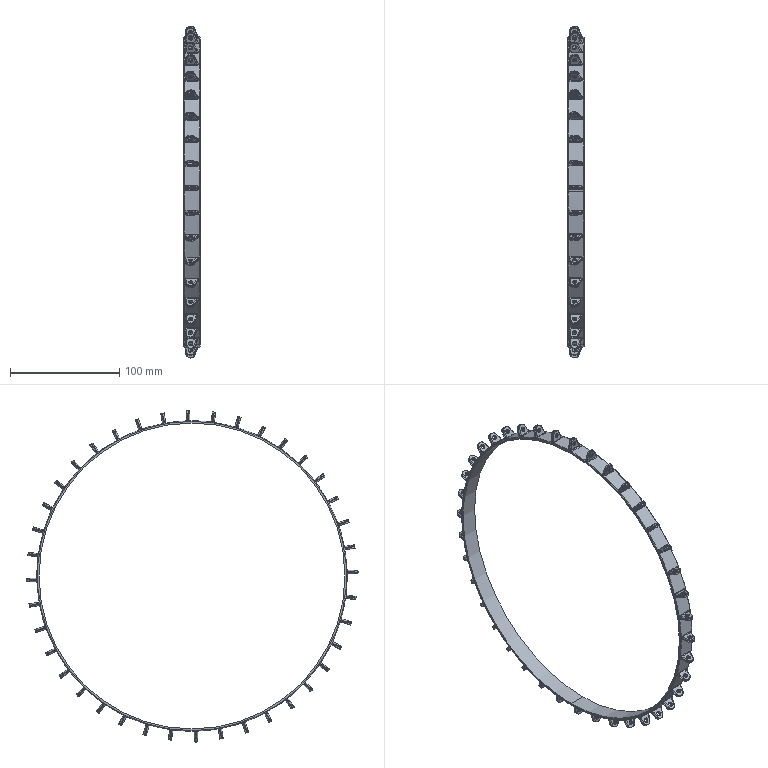Part | STEP file | Completa.sldasm-Part-278_Valor predeterminado | 1 solid | 1269 faces | box 15 x 303.98 x 303.98 mm | volume 32852 mm3 | cylinder 743 | spline 280 | plane 242 | torus 4 | commonest cylinder face diameters 2 x320 4 x160 1 x99 9 x80 10.4 x60 284.117 x22